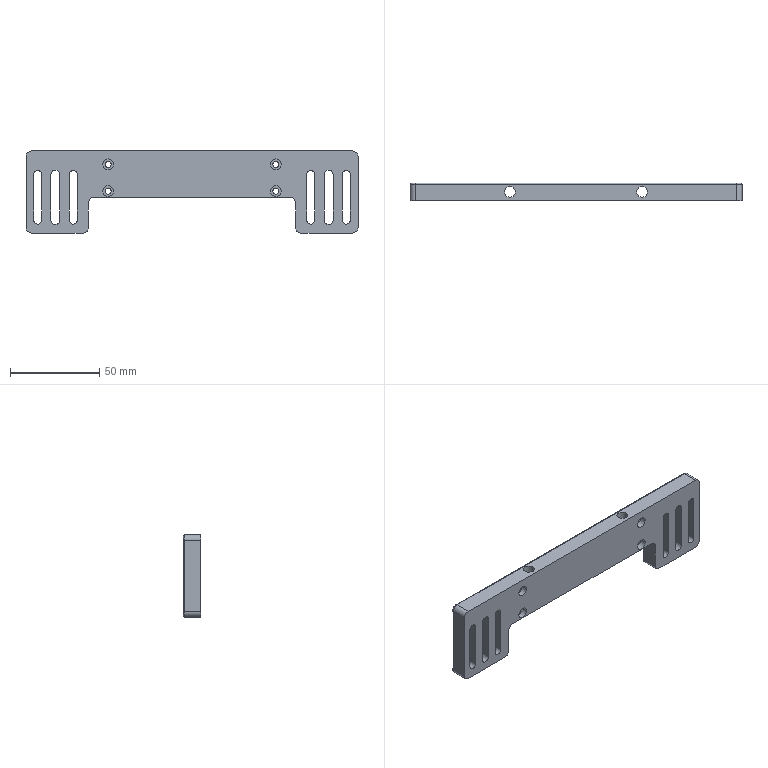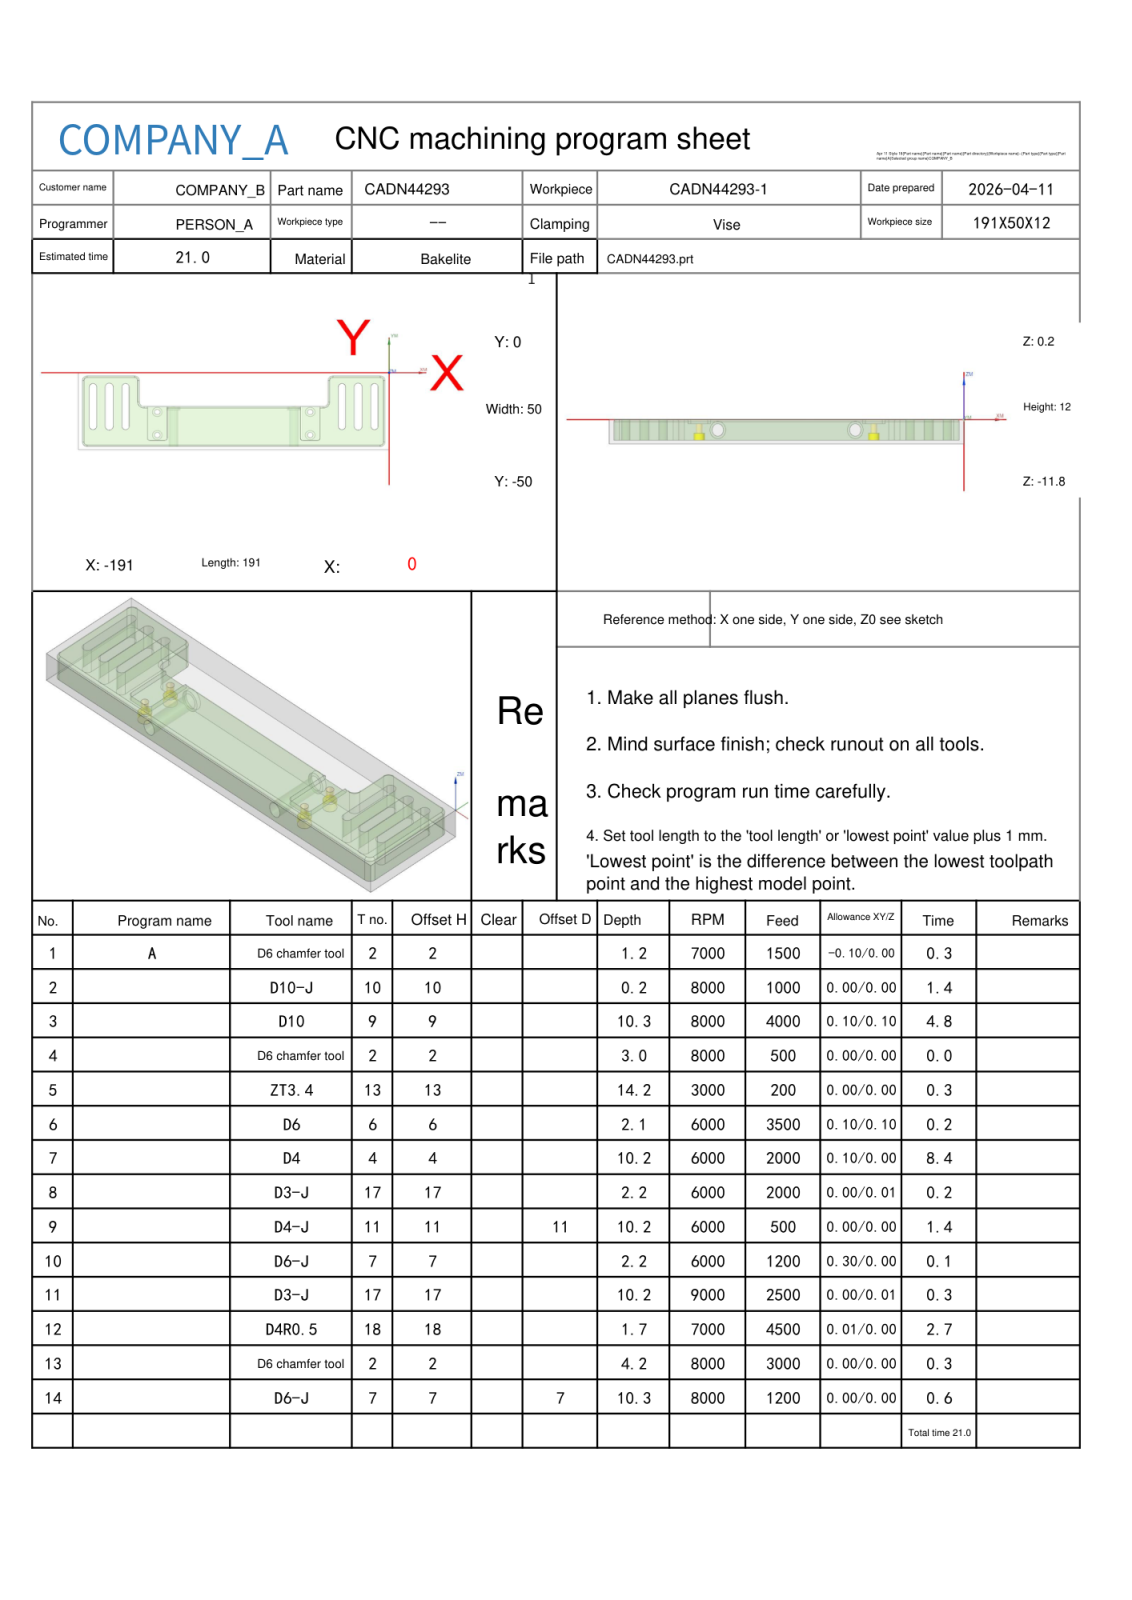NC program | NX | posted by the shop | part box 186 x 10 x 46 mm
Lines 3768 to 4733 of 7485:
N8 T17 M06
(D3-J  D=3. R=0. H=17 ce=0.00 di=0.01)
G00 G90 G54 X-146.473 Y-38.603 M03 S6000
G43 H17 Z20.
M08
Z.165
G01 X-146.479 Y-38.604 Z.097 F1600.
X-146.497 Y-38.606 Z.035
X-146.523 Y-38.61 Z-.02
X-146.558 Y-38.616 Z-.069
X-146.6 Y-38.625 Z-.112
X-146.647 Y-38.636 Z-.149
X-146.697 Y-38.649 Z-.181
X-146.75 Y-38.666 Z-.208
X-146.803 Y-38.685 Z-.23
X-146.855 Y-38.708 Z-.248
X-146.905 Y-38.733 Z-.262
X-146.951 Y-38.763 Z-.273
X-146.991 Y-38.796 Z-.28
X-147.025 Y-38.833 Z-.284
X-147.05 Y-38.875 Z-.285
Y-42.5 F2000.
X-143.425
X-143.396 Y-42.484 Z-.286
X-143.391 Y-42.439 Z-.288
X-143.408 Y-42.367 Z-.292
X-143.444 Y-42.272 Z-.298
X-143.498 Y-42.157 Z-.304
X-143.569 Y-42.025 Z-.312
X-143.75 Y-41.727 Z-.33
X-143.879 Y-41.534 Z-.342
X-144.103 Y-41.221 Z-.362
X-144.475 Y-40.765 Z-.394
X-144.881 Y-40.331 Z-.427
X-145.315 Y-39.925 Z-.461
X-145.771 Y-39.553 Z-.493
X-146.084 Y-39.329 Z-.513
X-146.277 Y-39.201 Z-.525
X-146.575 Y-39.019 Z-.543
X-146.707 Y-38.948 Z-.551
X-146.822 Y-38.894 Z-.557
X-146.917 Y-38.858 Z-.563
X-146.989 Y-38.841 Z-.567
X-147.034 Y-38.846 Z-.569
X-147.05 Y-38.875 Z-.57
Y-42.5
X-143.425
X-143.396 Y-42.484 Z-.571
X-143.391 Y-42.439 Z-.573
X-143.408 Y-42.367 Z-.577
X-143.444 Y-42.272 Z-.583
X-143.498 Y-42.157 Z-.589
X-143.569 Y-42.025 Z-.597
X-143.75 Y-41.727 Z-.615
X-143.879 Y-41.534 Z-.627
X-144.103 Y-41.221 Z-.647
X-144.475 Y-40.765 Z-.679
X-144.881 Y-40.331 Z-.712
X-145.315 Y-39.925 Z-.746
X-145.771 Y-39.553 Z-.778
X-146.084 Y-39.329 Z-.798
X-146.277 Y-39.201 Z-.81
X-146.575 Y-39.019 Z-.828
X-146.707 Y-38.948 Z-.836
X-146.822 Y-38.894 Z-.842
X-146.917 Y-38.858 Z-.848
X-146.989 Y-38.841 Z-.852
X-147.034 Y-38.846 Z-.854
X-147.05 Y-38.875 Z-.855
Y-42.5
X-143.425
X-143.396 Y-42.484 Z-.856
X-143.391 Y-42.439 Z-.858
X-143.407 Y-42.367 Z-.862
X-143.444 Y-42.272 Z-.868
X-143.498 Y-42.157 Z-.874
X-143.569 Y-42.025 Z-.882
X-143.75 Y-41.727 Z-.9
X-143.878 Y-41.534 Z-.912
X-144.102 Y-41.221 Z-.932
X-144.473 Y-40.765 Z-.964
X-144.879 Y-40.331 Z-.998
X-145.313 Y-39.925 Z-1.031
X-145.769 Y-39.553 Z-1.063
X-146.082 Y-39.329 Z-1.083
X-146.276 Y-39.2 Z-1.095
X-146.574 Y-39.019 Z-1.113
X-146.706 Y-38.948 Z-1.121
X-146.822 Y-38.894 Z-1.127
X-146.917 Y-38.858 Z-1.133
X-146.989 Y-38.841 Z-1.137
X-147.034 Y-38.846 Z-1.139
X-147.05 Y-38.875 Z-1.14
Y-42.5
X-143.425
X-143.396 Y-42.484 Z-1.141
X-143.391 Y-42.439 Z-1.143
X-143.407 Y-42.367 Z-1.147
X-143.444 Y-42.272 Z-1.153
X-143.498 Y-42.157 Z-1.159
X-143.569 Y-42.025 Z-1.167
X-143.75 Y-41.727 Z-1.185
X-143.878 Y-41.534 Z-1.197
X-144.102 Y-41.221 Z-1.217
X-144.473 Y-40.765 Z-1.249
X-144.879 Y-40.331 Z-1.283
X-145.313 Y-39.925 Z-1.316
X-145.769 Y-39.553 Z-1.348
X-146.082 Y-39.329 Z-1.368
X-146.276 Y-39.2 Z-1.38
X-146.574 Y-39.019 Z-1.398
X-146.706 Y-38.948 Z-1.406
X-146.822 Y-38.894 Z-1.412
X-146.917 Y-38.858 Z-1.418
X-146.989 Y-38.841 Z-1.422
X-147.034 Y-38.846 Z-1.424
X-147.05 Y-38.875 Z-1.425
Y-42.5
X-143.425
X-143.396 Y-42.484 Z-1.426
X-143.391 Y-42.439 Z-1.428
X-143.407 Y-42.367 Z-1.432
X-143.444 Y-42.272 Z-1.438
X-143.498 Y-42.157 Z-1.444
X-143.569 Y-42.025 Z-1.452
X-143.75 Y-41.727 Z-1.47
X-143.878 Y-41.534 Z-1.482
X-144.102 Y-41.221 Z-1.502
X-144.473 Y-40.765 Z-1.534
X-144.879 Y-40.331 Z-1.568
X-145.313 Y-39.925 Z-1.601
X-145.769 Y-39.553 Z-1.633
X-146.082 Y-39.329 Z-1.653
X-146.276 Y-39.2 Z-1.665
X-146.574 Y-39.019 Z-1.683
X-146.706 Y-38.948 Z-1.691
X-146.822 Y-38.894 Z-1.697
X-146.917 Y-38.858 Z-1.703
X-146.989 Y-38.841 Z-1.707
X-147.034 Y-38.846 Z-1.709
X-147.05 Y-38.875 Z-1.71
Y-42.5
X-143.425
X-143.396 Y-42.484 Z-1.711
X-143.391 Y-42.439 Z-1.713
X-143.407 Y-42.367 Z-1.717
X-143.444 Y-42.272 Z-1.723
X-143.498 Y-42.157 Z-1.729
X-143.569 Y-42.025 Z-1.737
X-143.75 Y-41.727 Z-1.755
X-143.878 Y-41.534 Z-1.767
X-144.102 Y-41.221 Z-1.787
X-144.473 Y-40.765 Z-1.819
X-144.879 Y-40.331 Z-1.853
X-145.313 Y-39.925 Z-1.886
X-145.769 Y-39.553 Z-1.918
X-146.082 Y-39.329 Z-1.938
X-146.276 Y-39.2 Z-1.95
X-146.574 Y-39.019 Z-1.968
X-146.706 Y-38.948 Z-1.976
X-146.822 Y-38.894 Z-1.982
X-146.917 Y-38.858 Z-1.988
X-146.989 Y-38.841 Z-1.992
X-147.034 Y-38.846 Z-1.994
X-147.05 Y-38.875 Z-1.995
Y-42.5
X-143.425
X-143.356 Y-42.487 Z-1.982
X-143.278 Y-42.453 Z-1.947
X-143.194 Y-42.403 Z-1.891
X-143.105 Y-42.343 Z-1.819
X-143.013 Y-42.279 Z-1.733
X-142.918 Y-42.217 Z-1.636
X-142.824 Y-42.163 Z-1.532
X-142.661 Y-42.099 Z-1.339
X-142.5 Y-42.078 Z-1.14
X-142.339 Y-42.099 Z-.941
X-142.176 Y-42.163 Z-.748
X-142.082 Y-42.217 Z-.644
X-141.987 Y-42.279 Z-.547
X-141.895 Y-42.343 Z-.461
X-141.806 Y-42.403 Z-.389
X-141.722 Y-42.453 Z-.333
X-141.644 Y-42.487 Z-.298
X-141.575 Y-42.5 Z-.285
X-137.95
Y-38.875
X-137.966 Y-38.846 Z-.286
X-138.011 Y-38.841 Z-.288
X-138.083 Y-38.858 Z-.292
X-138.178 Y-38.894 Z-.298
X-138.293 Y-38.948 Z-.304
X-138.425 Y-39.019 Z-.312
X-138.723 Y-39.201 Z-.33
X-138.916 Y-39.329 Z-.342
X-139.229 Y-39.553 Z-.362
X-139.685 Y-39.925 Z-.394
X-140.119 Y-40.331 Z-.428
X-140.525 Y-40.765 Z-.461
X-140.897 Y-41.221 Z-.493
X-141.121 Y-41.534 Z-.513
X-141.249 Y-41.727 Z-.525
X-141.431 Y-42.025 Z-.543
X-141.502 Y-42.157 Z-.551
X-141.556 Y-42.272 Z-.557
X-141.592 Y-42.367 Z-.563
X-141.609 Y-42.439 Z-.567
X-141.604 Y-42.484 Z-.569
X-141.575 Y-42.5 Z-.57
X-137.95
Y-38.875
X-137.966 Y-38.846 Z-.571
X-138.011 Y-38.841 Z-.573
X-138.083 Y-38.858 Z-.577
X-138.178 Y-38.894 Z-.583
X-138.293 Y-38.948 Z-.589
X-138.425 Y-39.019 Z-.597
X-138.723 Y-39.201 Z-.615
X-138.916 Y-39.329 Z-.627
X-139.229 Y-39.553 Z-.647
X-139.685 Y-39.925 Z-.679
X-140.119 Y-40.331 Z-.713
X-140.525 Y-40.765 Z-.746
X-140.897 Y-41.221 Z-.778
X-141.121 Y-41.534 Z-.798
X-141.249 Y-41.727 Z-.81
X-141.431 Y-42.025 Z-.828
X-141.502 Y-42.157 Z-.836
X-141.556 Y-42.272 Z-.842
X-141.592 Y-42.367 Z-.848
X-141.609 Y-42.439 Z-.852
X-141.604 Y-42.484 Z-.854
X-141.575 Y-42.5 Z-.855
X-137.95
Y-38.875
X-137.966 Y-38.846 Z-.856
X-138.011 Y-38.841 Z-.858
X-138.083 Y-38.858 Z-.862
X-138.178 Y-38.894 Z-.868
X-138.293 Y-38.948 Z-.874
X-138.425 Y-39.019 Z-.882
X-138.723 Y-39.201 Z-.9
X-138.916 Y-39.329 Z-.912
X-139.229 Y-39.553 Z-.932
X-139.685 Y-39.925 Z-.964
X-140.119 Y-40.331 Z-.998
X-140.525 Y-40.765 Z-1.031
X-140.897 Y-41.221 Z-1.063
X-141.121 Y-41.534 Z-1.083
X-141.249 Y-41.727 Z-1.095
X-141.431 Y-42.025 Z-1.113
X-141.502 Y-42.157 Z-1.121
X-141.556 Y-42.272 Z-1.127
X-141.592 Y-42.367 Z-1.133
X-141.609 Y-42.439 Z-1.137
X-141.604 Y-42.484 Z-1.139
X-141.575 Y-42.5 Z-1.14
X-137.95
Y-38.875
X-137.966 Y-38.846 Z-1.141
X-138.011 Y-38.841 Z-1.143
X-138.083 Y-38.858 Z-1.147
X-138.178 Y-38.894 Z-1.153
X-138.293 Y-38.948 Z-1.159
X-138.425 Y-39.019 Z-1.167
X-138.723 Y-39.201 Z-1.185
X-138.916 Y-39.329 Z-1.197
X-139.229 Y-39.553 Z-1.217
X-139.685 Y-39.925 Z-1.249
X-140.119 Y-40.331 Z-1.283
X-140.525 Y-40.765 Z-1.316
X-140.897 Y-41.221 Z-1.348
X-141.121 Y-41.534 Z-1.368
X-141.249 Y-41.727 Z-1.38
X-141.431 Y-42.025 Z-1.398
X-141.502 Y-42.157 Z-1.406
X-141.556 Y-42.272 Z-1.412
X-141.592 Y-42.367 Z-1.418
X-141.609 Y-42.439 Z-1.422
X-141.604 Y-42.484 Z-1.424
X-141.575 Y-42.5 Z-1.425
X-137.95
Y-38.875
X-137.966 Y-38.846 Z-1.426
X-138.011 Y-38.841 Z-1.428
X-138.083 Y-38.858 Z-1.432
X-138.178 Y-38.894 Z-1.438
X-138.293 Y-38.948 Z-1.444
X-138.425 Y-39.019 Z-1.452
X-138.723 Y-39.201 Z-1.47
X-138.916 Y-39.329 Z-1.482
X-139.229 Y-39.553 Z-1.502
X-139.685 Y-39.925 Z-1.534
X-140.119 Y-40.331 Z-1.568
X-140.525 Y-40.765 Z-1.601
X-140.897 Y-41.221 Z-1.633
X-141.121 Y-41.534 Z-1.653
X-141.249 Y-41.727 Z-1.665
X-141.431 Y-42.025 Z-1.683
X-141.502 Y-42.157 Z-1.691
X-141.556 Y-42.272 Z-1.697
X-141.592 Y-42.367 Z-1.703
X-141.609 Y-42.439 Z-1.707
X-141.604 Y-42.484 Z-1.709
X-141.575 Y-42.5 Z-1.71
X-137.95
Y-38.875
X-137.966 Y-38.846 Z-1.711
X-138.011 Y-38.841 Z-1.713
X-138.083 Y-38.858 Z-1.717
X-138.178 Y-38.894 Z-1.723
X-138.293 Y-38.948 Z-1.729
X-138.425 Y-39.019 Z-1.737
X-138.723 Y-39.201 Z-1.755
X-138.916 Y-39.329 Z-1.767
X-139.229 Y-39.553 Z-1.787
X-139.685 Y-39.925 Z-1.819
X-140.119 Y-40.331 Z-1.853
X-140.525 Y-40.765 Z-1.886
X-140.897 Y-41.221 Z-1.918
X-141.121 Y-41.534 Z-1.938
X-141.249 Y-41.727 Z-1.95
X-141.431 Y-42.025 Z-1.968
X-141.502 Y-42.157 Z-1.976
X-141.556 Y-42.272 Z-1.982
X-141.592 Y-42.367 Z-1.988
X-141.609 Y-42.439 Z-1.992
X-141.604 Y-42.484 Z-1.994
X-141.575 Y-42.5 Z-1.995
X-137.95
Y-38.875
X-137.96 Y-38.761 Z-1.993
X-137.986 Y-38.658 Z-1.986
X-138.028 Y-38.566 Z-1.975
X-138.082 Y-38.485 Z-1.957
X-138.144 Y-38.414 Z-1.934
X-138.214 Y-38.352 Z-1.904
X-138.288 Y-38.298 Z-1.867
X-138.362 Y-38.253 Z-1.821
X-138.436 Y-38.216 Z-1.768
X-138.506 Y-38.186 Z-1.706
X-138.568 Y-38.162 Z-1.635
X-138.622 Y-38.145 Z-1.553
X-138.664 Y-38.133 Z-1.462
X-138.69 Y-38.127 Z-1.359
X-138.7 Y-38.125 Z-1.245
G00 Z20.
X-52.593 Y-38.511
Z.187
G01 X-52.599 Y-38.513 Z.118 F1600.
X-52.615 Y-38.518 Z.056
X-52.641 Y-38.526 Z0.0
X-52.673 Y-38.538 Z-.051
X-52.712 Y-38.552 Z-.095
X-52.754 Y-38.57 Z-.135
X-52.799 Y-38.591 Z-.169
X-52.844 Y-38.616 Z-.198
X-52.889 Y-38.643 Z-.223
X-52.932 Y-38.674 Z-.243
X-52.97 Y-38.708 Z-.259
X-53.002 Y-38.745 Z-.27
X-53.028 Y-38.785 Z-.279
X-53.044 Y-38.828 Z-.283
X-53.05 Y-38.875 Z-.285
Y-42.5 F2000.
X-49.425
X-49.396 Y-42.484 Z-.286
X-49.391 Y-42.437 Z-.288
X-49.407 Y-42.364 Z-.292
X-49.444 Y-42.266 Z-.297
X-49.498 Y-42.148 Z-.303
X-49.569 Y-42.013 Z-.31
X-49.75 Y-41.707 Z-.327
X-49.878 Y-41.509 Z-.338
X-50.103 Y-41.186 Z-.357
X-50.397 Y-40.809 Z-.381
X-50.714 Y-40.446 Z-.406
X-51.05 Y-40.102 Z-.431
X-51.403 Y-39.782 Z-.457
X-51.77 Y-39.492 Z-.483
X-52.02 Y-39.317 Z-.501
X-52.185 Y-39.211 Z-.512
X-52.428 Y-39.067 Z-.529
X-52.574 Y-38.99 Z-.538
X-52.706 Y-38.926 Z-.547
X-52.822 Y-38.879 Z-.555
X-52.917 Y-38.848 Z-.561
X-52.989 Y-38.837 Z-.566
X-53.034 Y-38.845 Z-.569
X-53.05 Y-38.875 Z-.57
Y-42.5
X-49.425
X-49.396 Y-42.484 Z-.571
X-49.391 Y-42.437 Z-.573
X-49.408 Y-42.362 Z-.577
X-49.444 Y-42.263 Z-.582
X-49.499 Y-42.144 Z-.588
X-49.57 Y-42.007 Z-.595
X-49.752 Y-41.697 Z-.612
X-49.881 Y-41.495 Z-.624
X-50.106 Y-41.169 Z-.643
X-50.402 Y-40.785 Z-.667
X-50.72 Y-40.417 Z-.692
X-51.057 Y-40.069 Z-.718
X-51.411 Y-39.748 Z-.744
X-51.777 Y-39.46 Z-.77
X-52.026 Y-39.29 Z-.787
X-52.19 Y-39.187 Z-.798
X-52.432 Y-39.048 Z-.815
X-52.577 Y-38.974 Z-.824
X-52.709 Y-38.915 Z-.833
X-52.823 Y-38.871 Z-.84
X-52.918 Y-38.844 Z-.846
X-52.989 Y-38.835 Z-.851
X-53.034 Y-38.844 Z-.854
X-53.05 Y-38.875 Z-.855
Y-42.5
X-49.425
X-49.396 Y-42.483 Z-.856
X-49.391 Y-42.436 Z-.858
X-49.409 Y-42.36 Z-.862
X-49.446 Y-42.26 Z-.867
X-49.501 Y-42.139 Z-.873
X-49.573 Y-42. Z-.881
X-49.757 Y-41.687 Z-.898
X-49.887 Y-41.482 Z-.909
X-50.114 Y-41.151 Z-.929
X-50.412 Y-40.762 Z-.953
X-50.732 Y-40.388 Z-.978
X-51.071 Y-40.037 Z-1.004
X-51.425 Y-39.715 Z-1.031
X-51.79 Y-39.429 Z-1.057
X-51.958 Y-39.313 Z-1.068
X-52.125 Y-39.207 Z-1.08
X-52.286 Y-39.112 Z-1.09
X-52.44 Y-39.029 Z-1.101
X-52.584 Y-38.96 Z-1.11
X-52.714 Y-38.904 Z-1.118
X-52.827 Y-38.863 Z-1.126
X-52.92 Y-38.839 Z-1.132
X-52.99 Y-38.832 Z-1.136
X-53.035 Y-38.844 Z-1.139
X-53.05 Y-38.875 Z-1.14
Y-42.5
X-49.425
X-49.396 Y-42.483 Z-1.141
X-49.392 Y-42.435 Z-1.143
X-49.409 Y-42.359 Z-1.147
X-49.447 Y-42.258 Z-1.152
X-49.503 Y-42.136 Z-1.159
X-49.576 Y-41.995 Z-1.166
X-49.762 Y-41.678 Z-1.183
X-49.894 Y-41.471 Z-1.195
X-50.124 Y-41.135 Z-1.215
X-50.425 Y-40.741 Z-1.24
X-50.748 Y-40.363 Z-1.265
X-51.089 Y-40.009 Z-1.291
X-51.444 Y-39.686 Z-1.318
X-51.807 Y-39.402 Z-1.344
X-51.974 Y-39.288 Z-1.355
X-52.139 Y-39.184 Z-1.366
X-52.299 Y-39.092 Z-1.377
X-52.451 Y-39.013 Z-1.387
X-52.592 Y-38.946 Z-1.396
X-52.72 Y-38.894 Z-1.404
X-52.831 Y-38.857 Z-1.411
X-52.922 Y-38.835 Z-1.417
X-52.991 Y-38.83 Z-1.421
X-53.035 Y-38.843 Z-1.424
X-53.05 Y-38.875 Z-1.425
Y-42.5
X-49.425
X-49.396 Y-42.483 Z-1.426
X-49.392 Y-42.435 Z-1.428
X-49.411 Y-42.358 Z-1.432
X-49.449 Y-42.256 Z-1.438
X-49.507 Y-42.132 Z-1.444
X-49.63 Y-41.904 Z-1.456
X-49.843 Y-41.555 Z-1.476
X-50.092 Y-41.185 Z-1.497
X-50.389 Y-40.789 Z-1.522
X-50.657 Y-40.467 Z-1.543
X-50.938 Y-40.16 Z-1.565
X-51.229 Y-39.873 Z-1.587
X-51.527 Y-39.61 Z-1.609
X-51.829 Y-39.378 Z-1.631
X-52.011 Y-39.255 Z-1.643
X-52.189 Y-39.146 Z-1.655
X-52.36 Y-39.051 Z-1.666
X-52.521 Y-38.972 Z-1.677
X-52.667 Y-38.909 Z-1.686
X-52.795 Y-38.863 Z-1.694
X-52.901 Y-38.836 Z-1.701
X-52.981 Y-38.828 Z-1.706
X-53.032 Y-38.841 Z-1.709
X-53.05 Y-38.875 Z-1.71
Y-42.5
X-49.425
X-49.398 Y-42.486 Z-1.711
X-49.392 Y-42.444 Z-1.713
X-49.405 Y-42.379 Z-1.716
X-49.436 Y-42.291 Z-1.721
X-49.484 Y-42.184 Z-1.726
X-49.546 Y-42.06 Z-1.733
X-49.709 Y-41.776 Z-1.749
X-49.883 Y-41.501 Z-1.764
X-50.111 Y-41.168 Z-1.784
X-50.407 Y-40.777 Z-1.808
X-50.678 Y-40.452 Z-1.83
X-50.962 Y-40.142 Z-1.853
X-51.255 Y-39.854 Z-1.875
X-51.554 Y-39.592 Z-1.897
X-51.854 Y-39.361 Z-1.918
X-52.034 Y-39.239 Z-1.93
X-52.21 Y-39.131 Z-1.942
X-52.378 Y-39.039 Z-1.953
X-52.535 Y-38.962 Z-1.963
X-52.678 Y-38.901 Z-1.972
X-52.802 Y-38.858 Z-1.98
X-52.905 Y-38.833 Z-1.986
X-52.983 Y-38.827 Z-1.991
X-53.033 Y-38.84 Z-1.994
X-53.05 Y-38.875 Z-1.995
Y-42.5
X-49.425
X-49.356 Y-42.487 Z-1.982
X-49.278 Y-42.453 Z-1.947
X-49.194 Y-42.403 Z-1.891
X-49.105 Y-42.343 Z-1.819
X-49.013 Y-42.279 Z-1.733
X-48.918 Y-42.217 Z-1.636
X-48.824 Y-42.163 Z-1.532
X-48.661 Y-42.099 Z-1.339
X-48.5 Y-42.078 Z-1.14
X-48.339 Y-42.099 Z-.941
X-48.176 Y-42.163 Z-.748
X-48.082 Y-42.217 Z-.644
X-47.987 Y-42.279 Z-.547
X-47.895 Y-42.343 Z-.461
X-47.806 Y-42.403 Z-.389
X-47.722 Y-42.453 Z-.333
X-47.644 Y-42.487 Z-.298
X-47.575 Y-42.5 Z-.285
X-43.95
Y-38.875
X-43.966 Y-38.846 Z-.286
X-44.011 Y-38.841 Z-.288
X-44.083 Y-38.858 Z-.292
X-44.178 Y-38.894 Z-.298
X-44.293 Y-38.948 Z-.304
X-44.425 Y-39.019 Z-.312
X-44.723 Y-39.201 Z-.33
X-44.916 Y-39.329 Z-.342
X-45.229 Y-39.553 Z-.362
X-45.685 Y-39.925 Z-.394
X-46.119 Y-40.331 Z-.428
X-46.525 Y-40.765 Z-.461
X-46.897 Y-41.221 Z-.493
X-47.121 Y-41.534 Z-.513
X-47.249 Y-41.727 Z-.525
X-47.431 Y-42.025 Z-.543
X-47.502 Y-42.157 Z-.551
X-47.556 Y-42.272 Z-.557
X-47.592 Y-42.367 Z-.563
X-47.609 Y-42.439 Z-.567
X-47.604 Y-42.484 Z-.569
X-47.575 Y-42.5 Z-.57
X-43.95
Y-38.875
X-43.966 Y-38.846 Z-.571
X-44.011 Y-38.841 Z-.573
X-44.083 Y-38.858 Z-.577
X-44.178 Y-38.894 Z-.583
X-44.293 Y-38.948 Z-.589
X-44.425 Y-39.019 Z-.597
X-44.723 Y-39.201 Z-.615
X-44.916 Y-39.329 Z-.627
X-45.229 Y-39.553 Z-.647
X-45.685 Y-39.925 Z-.679
X-46.119 Y-40.331 Z-.713
X-46.525 Y-40.765 Z-.746
X-46.897 Y-41.221 Z-.778
X-47.121 Y-41.534 Z-.798
X-47.249 Y-41.727 Z-.81
X-47.431 Y-42.025 Z-.828
X-47.502 Y-42.157 Z-.836
X-47.556 Y-42.272 Z-.842
X-47.592 Y-42.367 Z-.848
X-47.609 Y-42.439 Z-.852
X-47.604 Y-42.484 Z-.854
X-47.575 Y-42.5 Z-.855
X-43.95
Y-38.875
X-43.966 Y-38.846 Z-.856
X-44.011 Y-38.841 Z-.858
X-44.083 Y-38.858 Z-.862
X-44.178 Y-38.894 Z-.868
X-44.293 Y-38.948 Z-.874
X-44.425 Y-39.019 Z-.882
X-44.723 Y-39.201 Z-.9
X-44.916 Y-39.329 Z-.912
X-45.229 Y-39.553 Z-.932
X-45.685 Y-39.925 Z-.964
X-46.119 Y-40.331 Z-.998
X-46.525 Y-40.765 Z-1.031
X-46.897 Y-41.221 Z-1.063
X-47.121 Y-41.534 Z-1.083
X-47.249 Y-41.727 Z-1.095
X-47.431 Y-42.025 Z-1.113
X-47.502 Y-42.157 Z-1.121
X-47.556 Y-42.272 Z-1.127
X-47.592 Y-42.367 Z-1.133
X-47.609 Y-42.439 Z-1.137
X-47.604 Y-42.484 Z-1.139
X-47.575 Y-42.5 Z-1.14
X-43.95
Y-38.875
X-43.966 Y-38.846 Z-1.141
X-44.011 Y-38.841 Z-1.143
X-44.083 Y-38.858 Z-1.147
X-44.178 Y-38.894 Z-1.153
X-44.293 Y-38.948 Z-1.159
X-44.425 Y-39.019 Z-1.167
X-44.723 Y-39.201 Z-1.185
X-44.916 Y-39.329 Z-1.197
X-45.229 Y-39.553 Z-1.217
X-45.685 Y-39.925 Z-1.249
X-46.119 Y-40.331 Z-1.283
X-46.525 Y-40.765 Z-1.316
X-46.897 Y-41.221 Z-1.348
X-47.121 Y-41.534 Z-1.368
X-47.249 Y-41.727 Z-1.38
X-47.431 Y-42.025 Z-1.398
X-47.502 Y-42.157 Z-1.406
X-47.556 Y-42.272 Z-1.412
X-47.592 Y-42.367 Z-1.418
X-47.609 Y-42.439 Z-1.422
X-47.604 Y-42.484 Z-1.424
X-47.575 Y-42.5 Z-1.425
X-43.95
Y-38.875
X-43.966 Y-38.846 Z-1.426
X-44.011 Y-38.841 Z-1.428
X-44.083 Y-38.858 Z-1.432
X-44.178 Y-38.894 Z-1.438
X-44.293 Y-38.948 Z-1.444
X-44.425 Y-39.019 Z-1.452
X-44.723 Y-39.201 Z-1.47
X-44.916 Y-39.329 Z-1.482
X-45.229 Y-39.553 Z-1.502
X-45.685 Y-39.925 Z-1.534
X-46.119 Y-40.331 Z-1.568
X-46.525 Y-40.765 Z-1.601
X-46.897 Y-41.221 Z-1.633
X-47.121 Y-41.534 Z-1.653
X-47.249 Y-41.727 Z-1.665
X-47.431 Y-42.025 Z-1.683
X-47.502 Y-42.157 Z-1.691
X-47.556 Y-42.272 Z-1.697
X-47.592 Y-42.367 Z-1.703
X-47.609 Y-42.439 Z-1.707
X-47.604 Y-42.484 Z-1.709
X-47.575 Y-42.5 Z-1.71
X-43.95
Y-38.875
X-43.966 Y-38.846 Z-1.711
X-44.011 Y-38.841 Z-1.713
X-44.083 Y-38.858 Z-1.717
X-44.178 Y-38.894 Z-1.723
X-44.293 Y-38.948 Z-1.729
X-44.425 Y-39.019 Z-1.737
X-44.723 Y-39.201 Z-1.755
X-44.916 Y-39.329 Z-1.767
X-45.229 Y-39.553 Z-1.787
X-45.685 Y-39.925 Z-1.819
X-46.119 Y-40.331 Z-1.853
X-46.525 Y-40.765 Z-1.886
X-46.897 Y-41.221 Z-1.918
X-47.121 Y-41.534 Z-1.938
X-47.249 Y-41.727 Z-1.95
X-47.431 Y-42.025 Z-1.968
X-47.502 Y-42.157 Z-1.976
X-47.556 Y-42.272 Z-1.982
X-47.592 Y-42.367 Z-1.988
X-47.609 Y-42.439 Z-1.992
X-47.604 Y-42.484 Z-1.994
X-47.575 Y-42.5 Z-1.995
X-43.95
Y-38.875
X-43.96 Y-38.761 Z-1.993
X-43.986 Y-38.658 Z-1.986
X-44.028 Y-38.566 Z-1.975
X-44.082 Y-38.485 Z-1.957
X-44.144 Y-38.414 Z-1.934
X-44.214 Y-38.351 Z-1.904
X-44.288 Y-38.298 Z-1.867
X-44.362 Y-38.253 Z-1.821
X-44.436 Y-38.216 Z-1.768
X-44.506 Y-38.186 Z-1.706
X-44.568 Y-38.162 Z-1.635
X-44.622 Y-38.145 Z-1.553
X-44.664 Y-38.133 Z-1.462
X-44.69 Y-38.127 Z-1.359
X-44.7 Y-38.125 Z-1.245
G00 Z20.
G91 G28 Z0.0
M05
M09
G91 G28 Z0.0
M01
N9 T11 M06
(D4-J  D=4. R=0. H=11 ce=0.00 di=0.00)
G00 G90 G54 X-18.75 Y-22.2 M03 S6000
G43 H11 Z20.
M08
Z-4.5
G01 Z-5. F500.
G41 D11
X-18.7
G03 X-18.5 Y-22. I0.0 J.2
G01 Y-9.25
G03 X-19. Y-8.75 I-.5 J0.0
X-19.5 Y-9.25 I0.0 J-.5
G01 Y-34.75
G03 X-19. Y-35.25 I.5 J0.0
X-18.5 Y-34.75 I0.0 J.5
G01 Y-22.
Y-21.5
G03 X-18.7 Y-21.3 I-.2 J0.0
G01 G40 X-18.75
Z-4.5
G00 Z.5
Y-22.2
Z-9.5
G01 Z-10.
G41 D11
X-18.7
G03 X-18.5 Y-22. I0.0 J.2
G01 Y-9.25
G03 X-19. Y-8.75 I-.5 J0.0
X-19.5 Y-9.25 I0.0 J-.5
G01 Y-34.75
G03 X-19. Y-35.25 I.5 J0.0
X-18.5 Y-34.75 I0.0 J.5
G01 Y-22.
Y-21.5
G03 X-18.7 Y-21.3 I-.2 J0.0
G01 G40 X-18.75
Z-9.5
G00 Z20.
X-172.25 Y-21.8
Z-4.5
G01 Z-5.
G41 D11
X-172.3
G03 X-172.5 Y-22. I0.0 J-.2
G01 Y-34.75
G03 X-172. Y-35.25 I.5 J0.0
X-171.5 Y-34.75 I0.0 J.5
G01 Y-9.25
G03 X-172. Y-8.75 I-.5 J0.0
X-172.5 Y-9.25 I0.0 J-.5
G01 Y-22.
Y-22.5
G03 X-172.3 Y-22.7 I.2 J0.0
G01 G40 X-172.25
Z-4.5
G00 Z.5
Y-21.8
Z-9.5
G01 Z-10.
G41 D11
X-172.3
G03 X-172.5 Y-22. I0.0 J-.2
G01 Y-34.75
G03 X-172. Y-35.25 I.5 J0.0
X-171.5 Y-34.75 I0.0 J.5
G01 Y-9.25
G03 X-172. Y-8.75 I-.5 J0.0
X-172.5 Y-9.25 I0.0 J-.5
G01 Y-22.
Y-22.5
G03 X-172.3 Y-22.7 I.2 J0.0
G01 G40 X-172.25
Z-9.5
G00 Z20.
G00 G90 X-9. Y-22.2 M03 S6000
Z20.
Z-4.5
G01 Z-5. F500.
G41 D11
X-8.95
G03 X-8.75 Y-22. I0.0 J.2
G01 Y-9.25
G03 X-9. Y-9. I-.25 J0.0
X-9.25 Y-9.25 I0.0 J-.25
G01 Y-34.75
G03 X-9. Y-35. I.25 J0.0
X-8.75 Y-34.75 I0.0 J.25
G01 Y-22.
Y-21.5
G03 X-8.95 Y-21.3 I-.2 J0.0
G01 G40 X-9.
Z-4.5
G00 Z1.
Y-22.2
Z-9.5
G01 Z-10.
G41 D11
X-8.95
G03 X-8.75 Y-22. I0.0 J.2
G01 Y-9.25
G03 X-9. Y-9. I-.25 J0.0
X-9.25 Y-9.25 I0.0 J-.25
G01 Y-34.75
G03 X-9. Y-35. I.25 J0.0
X-8.75 Y-34.75 I0.0 J.25
G01 Y-22.
Y-21.5
G03 X-8.95 Y-21.3 I-.2 J0.0
G01 G40 X-9.
Z-9.5
G00 Z20.
X-29. Y-22.2
Z-4.5
G01 Z-5.
G41 D11
X-28.95
G03 X-28.75 Y-22. I0.0 J.2
G01 Y-9.25
G03 X-29. Y-9. I-.25 J0.0
X-29.25 Y-9.25 I0.0 J-.25
G01 Y-34.75
G03 X-29. Y-35. I.25 J0.0
X-28.75 Y-34.75 I0.0 J.25
G01 Y-22.
Y-21.5
G03 X-28.95 Y-21.3 I-.2 J0.0
G01 G40 X-29.
Z-4.5
G00 Z1.
Y-22.2
Z-9.5
G01 Z-10.
G41 D11
X-28.95
G03 X-28.75 Y-22. I0.0 J.2
G01 Y-9.25
G03 X-29. Y-9. I-.25 J0.0
X-29.25 Y-9.25 I0.0 J-.25
G01 Y-34.75
G03 X-29. Y-35. I.25 J0.0
X-28.75 Y-34.75 I0.0 J.25
G01 Y-22.
Y-21.5
G03 X-28.95 Y-21.3 I-.2 J0.0
G01 G40 X-29.
Z-9.5
G00 Z20.
X-162. Y-22.2
Z-4.5
G01 Z-5.
G41 D11
X-161.95
G03 X-161.75 Y-22. I0.0 J.2
G01 Y-9.25
G03 X-162. Y-9. I-.25 J0.0
X-162.25 Y-9.25 I0.0 J-.25
G01 Y-34.75
G03 X-162. Y-35. I.25 J0.0
X-161.75 Y-34.75 I0.0 J.25
G01 Y-22.
Y-21.5
G03 X-161.95 Y-21.3 I-.2 J0.0
G01 G40 X-162.
Z-4.5
G00 Z1.
Y-22.2
Z-9.5
G01 Z-10.
G41 D11
X-161.95
G03 X-161.75 Y-22. I0.0 J.2
G01 Y-9.25
G03 X-162. Y-9. I-.25 J0.0
X-162.25 Y-9.25 I0.0 J-.25
G01 Y-34.75
G03 X-162. Y-35. I.25 J0.0
X-161.75 Y-34.75 I0.0 J.25
G01 Y-22.
Y-21.5
G03 X-161.95 Y-21.3 I-.2 J0.0
G01 G40 X-162.
Z-9.5
G00 Z20.
X-182. Y-21.8
Z-4.5
G01 Z-5.
G41 D11
X-182.05
G03 X-182.25 Y-22. I0.0 J-.2
G01 Y-34.75
G03 X-182. Y-35. I.25 J0.0
X-181.75 Y-34.75 I0.0 J.25
G01 Y-9.25
G03 X-182. Y-9. I-.25 J0.0
X-182.25 Y-9.25 I0.0 J-.25
G01 Y-22.
Y-22.5
G03 X-182.05 Y-22.7 I.2 J0.0
G01 G40 X-182.
Z-4.5
G00 Z1.
Y-21.8
Z-9.5
G01 Z-10.
G41 D11
X-182.05
G03 X-182.25 Y-22. I0.0 J-.2
G01 Y-34.75
G03 X-182. Y-35. I.25 J0.0
X-181.75 Y-34.75 I0.0 J.25
G01 Y-9.25
G03 X-182. Y-9. I-.25 J0.0
X-182.25 Y-9.25 I0.0 J-.25
G01 Y-22.
Y-22.5
G03 X-182.05 Y-22.7 I.2 J0.0
G01 G40 X-182.
Z-9.5
G00 Z20.
G91 G28 Z0.0
M05
M09
G91 G28 Z0.0
M01
N10 T07 M06
(D6-J  D=6. R=0. H=07 ce=0.30 di=0.00)
G00 G90 G54 X-51.25 Y-15.7 M03 S6000
G43 H07 Z20.
M08
Z-1.5
G01 Z-2. F1200.
Y-21.4
Y-40.7
X-45.75
Y-21.4
Y-15.7
Z-1.5
G00 Z20.
G00 G90 X-145.25 Y-15.7 M03 S6000
Z20.
Z-1.5
G01 Z-2. F1200.
Y-21.4
Y-40.7
X-139.75
Y-21.4
Y-15.7
Z-1.5
G00 Z20.
G91 G28 Z0.0
M05
M09
G91 G28 Z0.0
M01